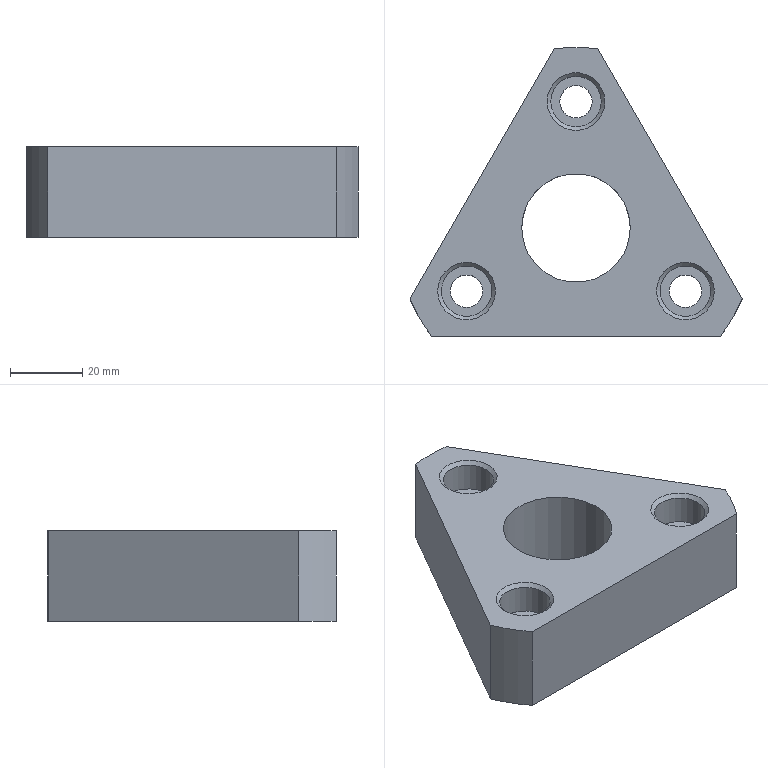CAM job | NX | 3-axis milling, drilling | part box 91.962 x 80 x 25 mm | stock box 101.962 x 86 x 26 mm
Tools:
number,name,description,diameter,corner_radius,flute_length,length,flutes
1,D25R0.8,Milling Tool-5 Parameters,25.0,0.8,50.0,75.0,2
2,D50R0.8,Milling Tool-5 Parameters,50.0,0.8,50.0,75.0,2
3,ZXZ,Milling Tool-5 Parameters,6.0,0.0,50.0,75.0,2
9,9.0ZT,Drilling Tool,9.0,0.0,35.0,50.0,2
8,18.0UZ,Milling Tool-5 Parameters,18.0,0.0,30.0,30.0,4
10,D10,Milling Tool-5 Parameters,10.0,0.0,50.0,75.0,2
11,D10JING,Milling Tool-5 Parameters,10.0,0.0,50.0,75.0,2
7,D6A45,Milling Tool-5 Parameters,6.0,0.0,3.0,3.0,2
Operations:
program,operation,operation_type,tool,method,geometry_group,spindle_rpm,surface_speed,feed_per_tooth,feed_cut,feed_plunge,cut_length_mm,path_length_mm,cut_time_min,machine_time_min
1,FLOOR_WALL,VolumeBased25DMillingOperation,D50R0.8,METHOD,A,1200.0,188.0,0.4167,1000.0,100.0,686.483,740.483,0.6865,0.6919
1,DRILLING,Operation,ZXZ,METHOD,A,3000.0,56.0,0.0417,250.0,0.0,16.0,231.953,0.064,0.0856
1,DRILLING_COPY,Operation,9.0ZT,METHOD,A,1000.0,28.0,0.1,200.0,0.0,96.612,380.615,0.4831,0.5115
1,DRILLING_COPY_COPY,Operation,18.0UZ,METHOD,A,400.0,22.0,0.0625,100.0,0.0,29.5,119.0,0.295,0.3039
1,ZLEVEL_PROFILE_1,ZLevelMilling,D50R0.8,METHOD,A,1197.0,188.0,0.6266,1500.0,100.0,22625.842,22709.842,15.084,15.092
1,ZLEVEL_PROFILE_COPY,ZLevelMilling,D25R0.8,METHOD,A,1600.0,50.0,0.5625,1800.0,1000.0,1495.329,1589.563,0.8536,0.8631
1,ZLEVEL_PROFILE,ZLevelMilling,D10,METHOD,A,3000.0,94.0,0.3,1800.0,1000.0,1974.784,2289.699,1.209,1.241
1,11,ZLevelMilling,D10JING,METHOD,A,5500.0,172.0,0.0909,1000.0,1000.0,625.038,733.289,0.625,0.6359
1,ZLEVEL_PROFILE_1_COPY_1_COPY,ZLevelMilling,D6A45,METHOD,A,9500.0,179.0,0.0526,1000.0,100.0,381.062,545.261,0.3811,0.3975
1,ZLEVEL_PROFILE_1_COPY_1_COPY_COPY,ZLevelMilling,D6A45,METHOD,A,9500.0,179.0,0.0526,1000.0,100.0,139.337,454.964,0.1393,0.1709
1,刀补11,ZLevelMilling,D10JING,METHOD,A,5500.0,172.0,0.0909,1000.0,1000.0,137.184,245.469,0.1372,0.148